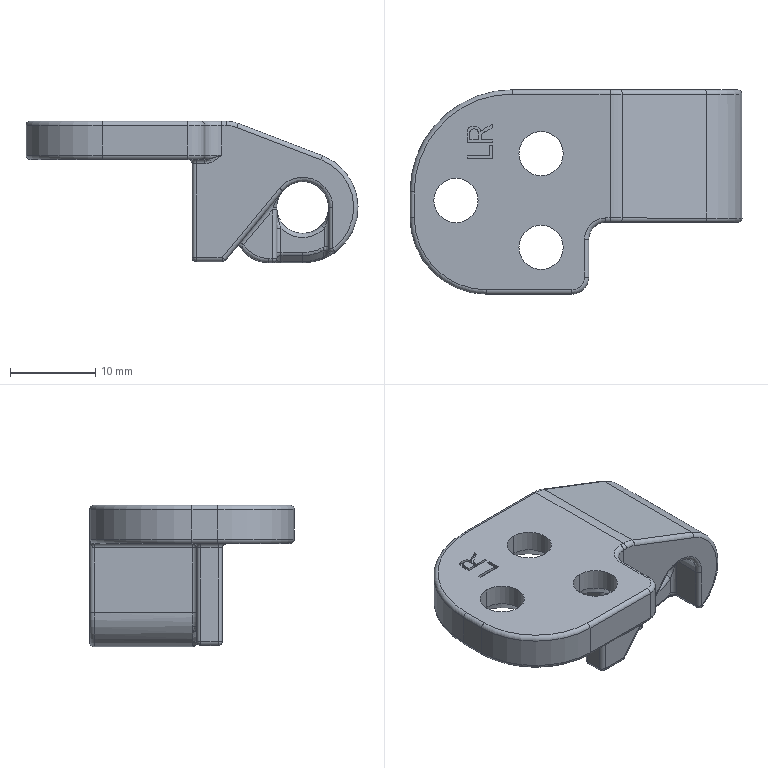Part | NX | features solid 2 | 1 solid | 145 faces | box 38.991 x 24 x 16.627 mm | volume 4278 mm3 | cylinder 52 | plane 38 | torus 22 | spline 19 | sphere 7 | cone 7 | commonest cylinder face diameters 1 x37 5.2 x6 4 x2 6.1 x2 8 x2 13 x1